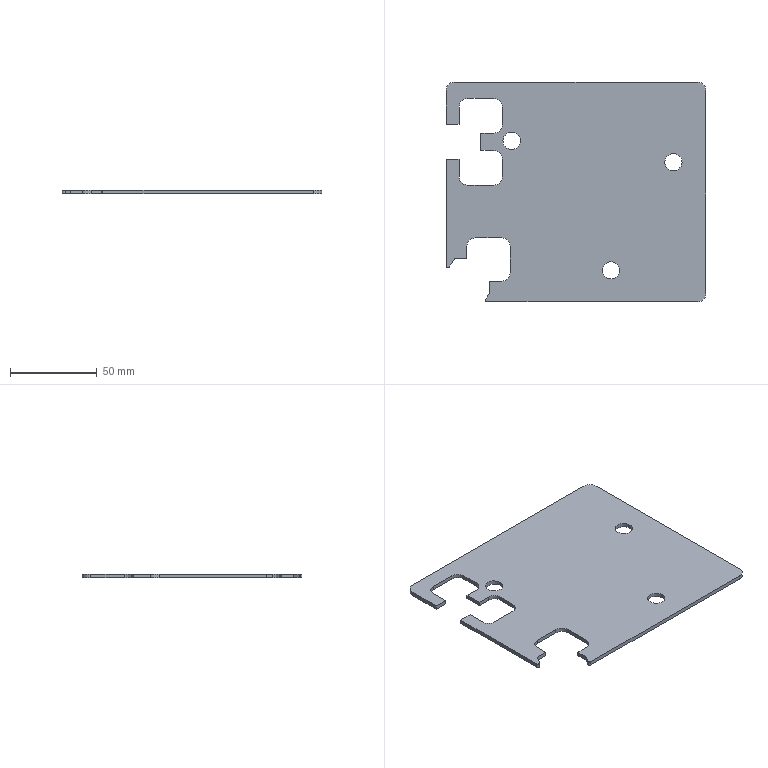Part | SolidWorks | features Fillet 1, FlatPattern 1, SMBaseFlange 1, SheetMetal 1 | 1 solid | 47 faces | box 150 x 127 x 2.3 mm | volume 37985 mm3 | plane 26 | cylinder 21 | commonest cylinder face diameters 10 x18 2 x3
STEP:
#1=CARTESIAN_POINT('',(-83.318,-80.043,2.3));
#2=VERTEX_POINT('',#1);
#3=CARTESIAN_POINT('',(-82.318,-81.043,2.3));
#4=VERTEX_POINT('',#3);
#5=CARTESIAN_POINT('',(-82.318,-80.043,2.3));
#6=DIRECTION('',(0.,0.,1.));
#7=DIRECTION('',(-1.,0.,0.));
#8=AXIS2_PLACEMENT_3D('',#5,#6,#7);
#9=CIRCLE('',#8,1.);
#10=EDGE_CURVE('',#2,#4,#9,.T.);
#11=ORIENTED_EDGE('',*,*,#10,.F.);
#12=CARTESIAN_POINT('',(-83.318,-80.043,0.));
#13=VERTEX_POINT('',#12);
#14=CARTESIAN_POINT('',(-83.318,-80.043,2.3));
#15=DIRECTION('',(0.,0.,-1.));
#16=VECTOR('',#15,1000.);
#17=LINE('',#14,#16);
#18=EDGE_CURVE('',#2,#13,#17,.T.);
#19=ORIENTED_EDGE('',*,*,#18,.T.);
#20=CARTESIAN_POINT('',(-82.318,-81.043,0.));
#21=VERTEX_POINT('',#20);
#22=CARTESIAN_POINT('',(-82.318,-80.043,0.));
#23=DIRECTION('',(0.,0.,-1.));
#24=DIRECTION('',(-1.,0.,0.));
#25=AXIS2_PLACEMENT_3D('',#22,#23,#24);
#26=CIRCLE('',#25,1.);
#27=EDGE_CURVE('',#21,#13,#26,.T.);
#28=ORIENTED_EDGE('',*,*,#27,.F.);
#29=CARTESIAN_POINT('',(-82.318,-81.043,2.3));
#30=DIRECTION('',(0.,0.,-1.));
#31=VECTOR('',#30,1000.);
#32=LINE('',#29,#31);
#33=EDGE_CURVE('',#4,#21,#32,.T.);
#34=ORIENTED_EDGE('',*,*,#33,.F.);
#35=EDGE_LOOP('',(#11,#19,#28,#34));
#36=FACE_OUTER_BOUND('',#35,.T.);
#37=CARTESIAN_POINT('',(-82.318,-80.043,2.3));
#38=DIRECTION('',(0.,0.,-1.));
#39=DIRECTION('',(-1.,0.,0.));
#40=AXIS2_PLACEMENT_3D('',#37,#38,#39);
#41=CYLINDRICAL_SURFACE('',#40,1.);
#42=ADVANCED_FACE('',(#36),#41,.T.);
#43=CARTESIAN_POINT('',(-15.703,-62.806,2.3));
#44=VERTEX_POINT('',#43);
#45=CARTESIAN_POINT('',(-5.703,-62.806,2.3));
#46=VERTEX_POINT('',#45);
#47=CARTESIAN_POINT('',(-10.703,-62.806,2.3));
#48=DIRECTION('',(0.,0.,1.));
#49=DIRECTION('',(1.,0.,0.));
#50=AXIS2_PLACEMENT_3D('',#47,#48,#49);
#51=CIRCLE('',#50,5.);
#52=EDGE_CURVE('',#44,#46,#51,.T.);
#53=ORIENTED_EDGE('',*,*,#52,.T.);
#54=CARTESIAN_POINT('',(-5.703,-62.806,0.));
#55=VERTEX_POINT('',#54);
#56=CARTESIAN_POINT('',(-5.703,-62.806,2.3));
#57=DIRECTION('',(0.,0.,-1.));
#58=VECTOR('',#57,1000.);
#59=LINE('',#56,#58);
#60=EDGE_CURVE('',#46,#55,#59,.T.);
#61=ORIENTED_EDGE('',*,*,#60,.T.);
#62=CARTESIAN_POINT('',(-15.703,-62.806,0.));
#63=VERTEX_POINT('',#62);
#64=CARTESIAN_POINT('',(-10.703,-62.806,0.));
#65=DIRECTION('',(0.,0.,1.));
#66=DIRECTION('',(1.,0.,0.));
#67=AXIS2_PLACEMENT_3D('',#64,#65,#66);
#68=CIRCLE('',#67,5.);
#69=EDGE_CURVE('',#63,#55,#68,.T.);
#70=ORIENTED_EDGE('',*,*,#69,.F.);
#71=CARTESIAN_POINT('',(-15.703,-62.806,2.3));
#72=DIRECTION('',(0.,0.,-1.));
#73=VECTOR('',#72,1000.);
#74=LINE('',#71,#73);
#75=EDGE_CURVE('',#44,#63,#74,.T.);
#76=ORIENTED_EDGE('',*,*,#75,.F.);
#77=EDGE_LOOP('',(#53,#61,#70,#76));
#78=FACE_OUTER_BOUND('',#77,.T.);
#79=CARTESIAN_POINT('',(-10.703,-62.806,2.3));
#80=DIRECTION('',(0.,0.,-1.));
#81=DIRECTION('',(-1.,0.,0.));
#82=AXIS2_PLACEMENT_3D('',#79,#80,#81);
#83=CYLINDRICAL_SURFACE('',#82,5.);
#84=ADVANCED_FACE('',(#78),#83,.F.);
#85=CARTESIAN_POINT('',(20.359,-0.3437,2.3));
#86=VERTEX_POINT('',#85);
#87=CARTESIAN_POINT('',(30.359,-0.3437,2.3));
#88=VERTEX_POINT('',#87);
#89=CARTESIAN_POINT('',(25.359,-0.3437,2.3));
#90=DIRECTION('',(0.,0.,1.));
#91=DIRECTION('',(1.,0.,0.));
#92=AXIS2_PLACEMENT_3D('',#89,#90,#91);
#93=CIRCLE('',#92,5.);
#94=EDGE_CURVE('',#86,#88,#93,.T.);
#95=ORIENTED_EDGE('',*,*,#94,.T.);
#96=CARTESIAN_POINT('',(30.359,-0.3437,0.));
#97=VERTEX_POINT('',#96);
#98=CARTESIAN_POINT('',(30.359,-0.3437,2.3));
#99=DIRECTION('',(0.,0.,-1.));
#100=VECTOR('',#99,1000.);
#101=LINE('',#98,#100);
#102=EDGE_CURVE('',#88,#97,#101,.T.);
#103=ORIENTED_EDGE('',*,*,#102,.T.);
#104=CARTESIAN_POINT('',(20.359,-0.3437,0.));
#105=VERTEX_POINT('',#104);
#106=CARTESIAN_POINT('',(25.359,-0.3437,0.));
#107=DIRECTION('',(0.,0.,1.));
#108=DIRECTION('',(1.,0.,0.));
#109=AXIS2_PLACEMENT_3D('',#106,#107,#108);
#110=CIRCLE('',#109,5.);
#111=EDGE_CURVE('',#105,#97,#110,.T.);
#112=ORIENTED_EDGE('',*,*,#111,.F.);
#113=CARTESIAN_POINT('',(20.359,-0.3437,2.3));
#114=DIRECTION('',(0.,0.,-1.));
#115=VECTOR('',#114,1000.);
#116=LINE('',#113,#115);
#117=EDGE_CURVE('',#86,#105,#116,.T.);
#118=ORIENTED_EDGE('',*,*,#117,.F.);
#119=EDGE_LOOP('',(#95,#103,#112,#118));
#120=FACE_OUTER_BOUND('',#119,.T.);
#121=CARTESIAN_POINT('',(25.359,-0.3437,2.3));
#122=DIRECTION('',(0.,0.,-1.));
#123=DIRECTION('',(-1.,0.,0.));
#124=AXIS2_PLACEMENT_3D('',#121,#122,#123);
#125=CYLINDRICAL_SURFACE('',#124,5.);
#126=ADVANCED_FACE('',(#120),#125,.F.);
#127=CARTESIAN_POINT('',(-73.07,11.957,2.3));
#128=VERTEX_POINT('',#127);
#129=CARTESIAN_POINT('',(-63.07,11.957,2.3));
#130=VERTEX_POINT('',#129);
#131=CARTESIAN_POINT('',(-68.07,11.957,2.3));
#132=DIRECTION('',(0.,0.,1.));
#133=DIRECTION('',(1.,0.,0.));
#134=AXIS2_PLACEMENT_3D('',#131,#132,#133);
#135=CIRCLE('',#134,5.);
#136=EDGE_CURVE('',#128,#130,#135,.T.);
#137=ORIENTED_EDGE('',*,*,#136,.T.);
#138=CARTESIAN_POINT('',(-63.07,11.957,0.));
#139=VERTEX_POINT('',#138);
#140=CARTESIAN_POINT('',(-63.07,11.957,2.3));
#141=DIRECTION('',(0.,0.,-1.));
#142=VECTOR('',#141,1000.);
#143=LINE('',#140,#142);
#144=EDGE_CURVE('',#130,#139,#143,.T.);
#145=ORIENTED_EDGE('',*,*,#144,.T.);
#146=CARTESIAN_POINT('',(-73.07,11.957,0.));
#147=VERTEX_POINT('',#146);
#148=CARTESIAN_POINT('',(-68.07,11.957,0.));
#149=DIRECTION('',(0.,0.,1.));
#150=DIRECTION('',(1.,0.,0.));
#151=AXIS2_PLACEMENT_3D('',#148,#149,#150);
#152=CIRCLE('',#151,5.);
#153=EDGE_CURVE('',#147,#139,#152,.T.);
#154=ORIENTED_EDGE('',*,*,#153,.F.);
#155=CARTESIAN_POINT('',(-73.07,11.957,2.3));
#156=DIRECTION('',(0.,0.,-1.));
#157=VECTOR('',#156,1000.);
#158=LINE('',#155,#157);
#159=EDGE_CURVE('',#128,#147,#158,.T.);
#160=ORIENTED_EDGE('',*,*,#159,.F.);
#161=EDGE_LOOP('',(#137,#145,#154,#160));
#162=FACE_OUTER_BOUND('',#161,.T.);
#163=CARTESIAN_POINT('',(-68.07,11.957,2.3));
#164=DIRECTION('',(0.,0.,-1.));
#165=DIRECTION('',(-1.,0.,0.));
#166=AXIS2_PLACEMENT_3D('',#163,#164,#165);
#167=CYLINDRICAL_SURFACE('',#166,5.);
#168=ADVANCED_FACE('',(#162),#167,.F.);
#169=CARTESIAN_POINT('',(-80.903,-76.043,2.3));
#170=VERTEX_POINT('',#169);
#171=CARTESIAN_POINT('',(-83.155,-79.497,2.3));
#172=VERTEX_POINT('',#171);
#173=CARTESIAN_POINT('',(-84.164,-81.043,2.3));
#174=DIRECTION('',(-0.5463,-0.8376,0.));
#175=VECTOR('',#174,1000.);
#176=LINE('',#173,#175);
#177=EDGE_CURVE('',#170,#172,#176,.T.);
#178=ORIENTED_EDGE('',*,*,#177,.T.);
#179=CARTESIAN_POINT('',(-82.318,-80.043,2.3));
#180=DIRECTION('',(0.,0.,1.));
#181=DIRECTION('',(-1.,0.,0.));
#182=AXIS2_PLACEMENT_3D('',#179,#180,#181);
#183=CIRCLE('',#182,1.);
#184=EDGE_CURVE('',#172,#2,#183,.T.);
#185=ORIENTED_EDGE('',*,*,#184,.T.);
#186=ORIENTED_EDGE('',*,*,#10,.T.);
#187=CARTESIAN_POINT('',(39.097,-81.043,2.3));
#188=VERTEX_POINT('',#187);
#189=CARTESIAN_POINT('',(-80.903,-81.043,2.3));
#190=DIRECTION('',(1.,0.,0.));
#191=VECTOR('',#190,1000.);
#192=LINE('',#189,#191);
#193=EDGE_CURVE('',#4,#188,#192,.T.);
#194=ORIENTED_EDGE('',*,*,#193,.T.);
#195=CARTESIAN_POINT('',(44.097,-76.043,2.3));
#196=VERTEX_POINT('',#195);
#197=CARTESIAN_POINT('',(39.097,-76.043,2.3));
#198=DIRECTION('',(0.,0.,1.));
#199=DIRECTION('',(-1.,0.,0.));
#200=AXIS2_PLACEMENT_3D('',#197,#198,#199);
#201=CIRCLE('',#200,5.);
#202=EDGE_CURVE('',#188,#196,#201,.T.);
#203=ORIENTED_EDGE('',*,*,#202,.T.);
#204=CARTESIAN_POINT('',(44.097,40.957,2.3));
#205=VERTEX_POINT('',#204);
#206=CARTESIAN_POINT('',(44.097,-76.043,2.3));
#207=DIRECTION('',(0.,1.,0.));
#208=VECTOR('',#207,1000.);
#209=LINE('',#206,#208);
#210=EDGE_CURVE('',#196,#205,#209,.T.);
#211=ORIENTED_EDGE('',*,*,#210,.T.);
#212=CARTESIAN_POINT('',(39.097,45.957,2.3));
#213=VERTEX_POINT('',#212);
#214=CARTESIAN_POINT('',(39.097,40.957,2.3));
#215=DIRECTION('',(0.,0.,1.));
#216=DIRECTION('',(1.,0.,0.));
#217=AXIS2_PLACEMENT_3D('',#214,#215,#216);
#218=CIRCLE('',#217,5.);
#219=EDGE_CURVE('',#205,#213,#218,.T.);
#220=ORIENTED_EDGE('',*,*,#219,.T.);
#221=CARTESIAN_POINT('',(-100.903,45.957,2.3));
#222=VERTEX_POINT('',#221);
#223=CARTESIAN_POINT('',(39.097,45.957,2.3));
#224=DIRECTION('',(-1.,0.,0.));
#225=VECTOR('',#224,1000.);
#226=LINE('',#223,#225);
#227=EDGE_CURVE('',#213,#222,#226,.T.);
#228=ORIENTED_EDGE('',*,*,#227,.T.);
#229=CARTESIAN_POINT('',(-105.903,40.957,2.3));
#230=VERTEX_POINT('',#229);
#231=CARTESIAN_POINT('',(-100.903,40.957,2.3));
#232=DIRECTION('',(0.,0.,1.));
#233=DIRECTION('',(1.,0.,0.));
#234=AXIS2_PLACEMENT_3D('',#231,#232,#233);
#235=CIRCLE('',#234,5.);
#236=EDGE_CURVE('',#222,#230,#235,.T.);
#237=ORIENTED_EDGE('',*,*,#236,.T.);
#238=CARTESIAN_POINT('',(-105.903,21.457,2.3));
#239=VERTEX_POINT('',#238);
#240=CARTESIAN_POINT('',(-105.903,40.957,2.3));
#241=DIRECTION('',(0.,-1.,0.));
#242=VECTOR('',#241,1000.);
#243=LINE('',#240,#242);
#244=EDGE_CURVE('',#230,#239,#243,.T.);
#245=ORIENTED_EDGE('',*,*,#244,.T.);
#246=CARTESIAN_POINT('',(-98.403,21.457,2.3));
#247=VERTEX_POINT('',#246);
#248=CARTESIAN_POINT('',(-105.903,21.457,2.3));
#249=DIRECTION('',(1.,0.,0.));
#250=VECTOR('',#249,1000.);
#251=LINE('',#248,#250);
#252=EDGE_CURVE('',#239,#247,#251,.T.);
#253=ORIENTED_EDGE('',*,*,#252,.T.);
#254=CARTESIAN_POINT('',(-98.403,31.457,2.3));
#255=VERTEX_POINT('',#254);
#256=CARTESIAN_POINT('',(-98.403,21.457,2.3));
#257=DIRECTION('',(0.,1.,0.));
#258=VECTOR('',#257,1000.);
#259=LINE('',#256,#258);
#260=EDGE_CURVE('',#247,#255,#259,.T.);
#261=ORIENTED_EDGE('',*,*,#260,.T.);
#262=CARTESIAN_POINT('',(-93.403,36.457,2.3));
#263=VERTEX_POINT('',#262);
#264=CARTESIAN_POINT('',(-93.403,31.457,2.3));
#265=DIRECTION('',(0.,0.,-1.));
#266=DIRECTION('',(-1.,0.,0.));
#267=AXIS2_PLACEMENT_3D('',#264,#265,#266);
#268=CIRCLE('',#267,5.);
#269=EDGE_CURVE('',#255,#263,#268,.T.);
#270=ORIENTED_EDGE('',*,*,#269,.T.);
#271=CARTESIAN_POINT('',(-78.403,36.457,2.3));
#272=VERTEX_POINT('',#271);
#273=CARTESIAN_POINT('',(-93.403,36.457,2.3));
#274=DIRECTION('',(1.,0.,0.));
#275=VECTOR('',#274,1000.);
#276=LINE('',#273,#275);
#277=EDGE_CURVE('',#263,#272,#276,.T.);
#278=ORIENTED_EDGE('',*,*,#277,.T.);
#279=CARTESIAN_POINT('',(-73.403,31.457,2.3));
#280=VERTEX_POINT('',#279);
#281=CARTESIAN_POINT('',(-78.403,31.457,2.3));
#282=DIRECTION('',(0.,0.,-1.));
#283=DIRECTION('',(-1.,0.,0.));
#284=AXIS2_PLACEMENT_3D('',#281,#282,#283);
#285=CIRCLE('',#284,5.);
#286=EDGE_CURVE('',#272,#280,#285,.T.);
#287=ORIENTED_EDGE('',*,*,#286,.T.);
#288=CARTESIAN_POINT('',(-73.403,21.457,2.3));
#289=VERTEX_POINT('',#288);
#290=CARTESIAN_POINT('',(-73.403,31.457,2.3));
#291=DIRECTION('',(0.,-1.,0.));
#292=VECTOR('',#291,1000.);
#293=LINE('',#290,#292);
#294=EDGE_CURVE('',#280,#289,#293,.T.);
#295=ORIENTED_EDGE('',*,*,#294,.T.);
#296=CARTESIAN_POINT('',(-78.403,16.457,2.3));
#297=VERTEX_POINT('',#296);
#298=CARTESIAN_POINT('',(-78.403,21.457,2.3));
#299=DIRECTION('',(0.,0.,-1.));
#300=DIRECTION('',(-1.,0.,0.));
#301=AXIS2_PLACEMENT_3D('',#298,#299,#300);
#302=CIRCLE('',#301,5.);
#303=EDGE_CURVE('',#289,#297,#302,.T.);
#304=ORIENTED_EDGE('',*,*,#303,.T.);
#305=CARTESIAN_POINT('',(-85.903,16.457,2.3));
#306=VERTEX_POINT('',#305);
#307=CARTESIAN_POINT('',(-78.403,16.457,2.3));
#308=DIRECTION('',(-1.,0.,0.));
#309=VECTOR('',#308,1000.);
#310=LINE('',#307,#309);
#311=EDGE_CURVE('',#297,#306,#310,.T.);
#312=ORIENTED_EDGE('',*,*,#311,.T.);
#313=CARTESIAN_POINT('',(-85.903,6.457,2.3));
#314=VERTEX_POINT('',#313);
#315=CARTESIAN_POINT('',(-85.903,16.457,2.3));
#316=DIRECTION('',(0.,-1.,0.));
#317=VECTOR('',#316,1000.);
#318=LINE('',#315,#317);
#319=EDGE_CURVE('',#306,#314,#318,.T.);
#320=ORIENTED_EDGE('',*,*,#319,.T.);
#321=CARTESIAN_POINT('',(-78.403,6.457,2.3));
#322=VERTEX_POINT('',#321);
#323=CARTESIAN_POINT('',(-85.903,6.457,2.3));
#324=DIRECTION('',(1.,0.,0.));
#325=VECTOR('',#324,1000.);
#326=LINE('',#323,#325);
#327=EDGE_CURVE('',#314,#322,#326,.T.);
#328=ORIENTED_EDGE('',*,*,#327,.T.);
#329=CARTESIAN_POINT('',(-73.403,1.457,2.3));
#330=VERTEX_POINT('',#329);
#331=CARTESIAN_POINT('',(-78.403,1.457,2.3));
#332=DIRECTION('',(0.,0.,-1.));
#333=DIRECTION('',(-1.,0.,0.));
#334=AXIS2_PLACEMENT_3D('',#331,#332,#333);
#335=CIRCLE('',#334,5.);
#336=EDGE_CURVE('',#322,#330,#335,.T.);
#337=ORIENTED_EDGE('',*,*,#336,.T.);
#338=CARTESIAN_POINT('',(-73.403,-8.543,2.3));
#339=VERTEX_POINT('',#338);
#340=CARTESIAN_POINT('',(-73.403,1.457,2.3));
#341=DIRECTION('',(0.,-1.,0.));
#342=VECTOR('',#341,1000.);
#343=LINE('',#340,#342);
#344=EDGE_CURVE('',#330,#339,#343,.T.);
#345=ORIENTED_EDGE('',*,*,#344,.T.);
#346=CARTESIAN_POINT('',(-78.403,-13.543,2.3));
#347=VERTEX_POINT('',#346);
#348=CARTESIAN_POINT('',(-78.403,-8.543,2.3));
#349=DIRECTION('',(0.,0.,-1.));
#350=DIRECTION('',(-1.,0.,0.));
#351=AXIS2_PLACEMENT_3D('',#348,#349,#350);
#352=CIRCLE('',#351,5.);
#353=EDGE_CURVE('',#339,#347,#352,.T.);
#354=ORIENTED_EDGE('',*,*,#353,.T.);
#355=CARTESIAN_POINT('',(-93.403,-13.543,2.3));
#356=VERTEX_POINT('',#355);
#357=CARTESIAN_POINT('',(-78.403,-13.543,2.3));
#358=DIRECTION('',(-1.,0.,0.));
#359=VECTOR('',#358,1000.);
#360=LINE('',#357,#359);
#361=EDGE_CURVE('',#347,#356,#360,.T.);
#362=ORIENTED_EDGE('',*,*,#361,.T.);
#363=CARTESIAN_POINT('',(-98.403,-8.543,2.3));
#364=VERTEX_POINT('',#363);
#365=CARTESIAN_POINT('',(-93.403,-8.543,2.3));
#366=DIRECTION('',(0.,0.,-1.));
#367=DIRECTION('',(-1.,0.,0.));
#368=AXIS2_PLACEMENT_3D('',#365,#366,#367);
#369=CIRCLE('',#368,5.);
#370=EDGE_CURVE('',#356,#364,#369,.T.);
#371=ORIENTED_EDGE('',*,*,#370,.T.);
#372=CARTESIAN_POINT('',(-98.403,1.457,2.3));
#373=VERTEX_POINT('',#372);
#374=CARTESIAN_POINT('',(-98.403,-8.543,2.3));
#375=DIRECTION('',(0.,1.,0.));
#376=VECTOR('',#375,1000.);
#377=LINE('',#374,#376);
#378=EDGE_CURVE('',#364,#373,#377,.T.);
#379=ORIENTED_EDGE('',*,*,#378,.T.);
#380=CARTESIAN_POINT('',(-105.903,1.457,2.3));
#381=VERTEX_POINT('',#380);
#382=CARTESIAN_POINT('',(-98.403,1.457,2.3));
#383=DIRECTION('',(-1.,0.,0.));
#384=VECTOR('',#383,1000.);
#385=LINE('',#382,#384);
#386=EDGE_CURVE('',#373,#381,#385,.T.);
#387=ORIENTED_EDGE('',*,*,#386,.T.);
#388=CARTESIAN_POINT('',(-105.903,-60.346,2.3));
#389=VERTEX_POINT('',#388);
#390=CARTESIAN_POINT('',(-105.903,1.457,2.3));
#391=DIRECTION('',(0.,-1.,0.));
#392=VECTOR('',#391,1000.);
#393=LINE('',#390,#392);
#394=EDGE_CURVE('',#381,#389,#393,.T.);
#395=ORIENTED_EDGE('',*,*,#394,.T.);
#396=CARTESIAN_POINT('',(-104.065,-60.892,2.3));
#397=VERTEX_POINT('',#396);
#398=CARTESIAN_POINT('',(-104.903,-60.346,2.3));
#399=DIRECTION('',(0.,0.,1.));
#400=DIRECTION('',(-1.,0.,0.));
#401=AXIS2_PLACEMENT_3D('',#398,#399,#400);
#402=CIRCLE('',#401,1.);
#403=EDGE_CURVE('',#389,#397,#402,.T.);
#404=ORIENTED_EDGE('',*,*,#403,.T.);
#405=CARTESIAN_POINT('',(-100.903,-56.043,2.3));
#406=VERTEX_POINT('',#405);
#407=CARTESIAN_POINT('',(-105.903,-63.71,2.3));
#408=DIRECTION('',(0.5463,0.8376,0.));
#409=VECTOR('',#408,1000.);
#410=LINE('',#407,#409);
#411=EDGE_CURVE('',#397,#406,#410,.T.);
#412=ORIENTED_EDGE('',*,*,#411,.T.);
#413=CARTESIAN_POINT('',(-93.903,-56.043,2.3));
#414=VERTEX_POINT('',#413);
#415=CARTESIAN_POINT('',(-93.903,-56.043,2.3));
#416=DIRECTION('',(1.,0.,0.));
#417=VECTOR('',#416,1000.);
#418=LINE('',#415,#417);
#419=EDGE_CURVE('',#406,#414,#418,.T.);
#420=ORIENTED_EDGE('',*,*,#419,.T.);
#421=CARTESIAN_POINT('',(-93.903,-49.043,2.3));
#422=VERTEX_POINT('',#421);
#423=CARTESIAN_POINT('',(-93.903,-56.043,2.3));
#424=DIRECTION('',(0.,1.,0.));
#425=VECTOR('',#424,1000.);
#426=LINE('',#423,#425);
#427=EDGE_CURVE('',#414,#422,#426,.T.);
#428=ORIENTED_EDGE('',*,*,#427,.T.);
#429=CARTESIAN_POINT('',(-88.903,-44.043,2.3));
#430=VERTEX_POINT('',#429);
#431=CARTESIAN_POINT('',(-88.903,-49.043,2.3));
#432=DIRECTION('',(0.,0.,-1.));
#433=DIRECTION('',(-1.,0.,0.));
#434=AXIS2_PLACEMENT_3D('',#431,#432,#433);
#435=CIRCLE('',#434,5.);
#436=EDGE_CURVE('',#422,#430,#435,.T.);
#437=ORIENTED_EDGE('',*,*,#436,.T.);
#438=CARTESIAN_POINT('',(-73.903,-44.043,2.3));
#439=VERTEX_POINT('',#438);
#440=CARTESIAN_POINT('',(-88.903,-44.043,2.3));
#441=DIRECTION('',(1.,0.,0.));
#442=VECTOR('',#441,1000.);
#443=LINE('',#440,#442);
#444=EDGE_CURVE('',#430,#439,#443,.T.);
#445=ORIENTED_EDGE('',*,*,#444,.T.);
#446=CARTESIAN_POINT('',(-68.903,-49.043,2.3));
#447=VERTEX_POINT('',#446);
#448=CARTESIAN_POINT('',(-73.903,-49.043,2.3));
#449=DIRECTION('',(0.,0.,-1.));
#450=DIRECTION('',(-1.,0.,0.));
#451=AXIS2_PLACEMENT_3D('',#448,#449,#450);
#452=CIRCLE('',#451,5.);
#453=EDGE_CURVE('',#439,#447,#452,.T.);
#454=ORIENTED_EDGE('',*,*,#453,.T.);
#455=CARTESIAN_POINT('',(-68.903,-64.043,2.3));
#456=VERTEX_POINT('',#455);
#457=CARTESIAN_POINT('',(-68.903,-49.043,2.3));
#458=DIRECTION('',(0.,-1.,0.));
#459=VECTOR('',#458,1000.);
#460=LINE('',#457,#459);
#461=EDGE_CURVE('',#447,#456,#460,.T.);
#462=ORIENTED_EDGE('',*,*,#461,.T.);
#463=CARTESIAN_POINT('',(-73.903,-69.043,2.3));
#464=VERTEX_POINT('',#463);
#465=CARTESIAN_POINT('',(-73.903,-64.043,2.3));
#466=DIRECTION('',(0.,0.,-1.));
#467=DIRECTION('',(-1.,0.,0.));
#468=AXIS2_PLACEMENT_3D('',#465,#466,#467);
#469=CIRCLE('',#468,5.);
#470=EDGE_CURVE('',#456,#464,#469,.T.);
#471=ORIENTED_EDGE('',*,*,#470,.T.);
#472=CARTESIAN_POINT('',(-80.903,-69.043,2.3));
#473=VERTEX_POINT('',#472);
#474=CARTESIAN_POINT('',(-73.903,-69.043,2.3));
#475=DIRECTION('',(-1.,0.,0.));
#476=VECTOR('',#475,1000.);
#477=LINE('',#474,#476);
#478=EDGE_CURVE('',#464,#473,#477,.T.);
#479=ORIENTED_EDGE('',*,*,#478,.T.);
#480=CARTESIAN_POINT('',(-80.903,-69.043,2.3));
#481=DIRECTION('',(0.,-1.,0.));
#482=VECTOR('',#481,1000.);
#483=LINE('',#480,#482);
#484=EDGE_CURVE('',#473,#170,#483,.T.);
#485=ORIENTED_EDGE('',*,*,#484,.T.);
#486=EDGE_LOOP('',(#178,#185,#186,#194,#203,#211,#220,#228,#237,#245,#253,#261,#270,#278,#287,#295,#304,#312,#320,#328,#337,#345,#354,#362,#371,#379,#387,#395,#404,#412,#420,#428,#437,#445,#454,#462,#471,#479,#485));
#487=FACE_OUTER_BOUND('',#486,.T.);
#488=ORIENTED_EDGE('',*,*,#136,.F.);
#489=CARTESIAN_POINT('',(-68.07,11.957,2.3));
#490=DIRECTION('',(0.,0.,1.));
#491=DIRECTION('',(1.,0.,0.));
#492=AXIS2_PLACEMENT_3D('',#489,#490,#491);
#493=CIRCLE('',#492,5.);
#494=EDGE_CURVE('',#130,#128,#493,.T.);
#495=ORIENTED_EDGE('',*,*,#494,.F.);
#496=EDGE_LOOP('',(#488,#495));
#497=FACE_BOUND('',#496,.T.);
#498=ORIENTED_EDGE('',*,*,#94,.F.);
#499=CARTESIAN_POINT('',(25.359,-0.3437,2.3));
#500=DIRECTION('',(0.,0.,1.));
#501=DIRECTION('',(1.,0.,0.));
#502=AXIS2_PLACEMENT_3D('',#499,#500,#501);
#503=CIRCLE('',#502,5.);
#504=EDGE_CURVE('',#88,#86,#503,.T.);
#505=ORIENTED_EDGE('',*,*,#504,.F.);
#506=EDGE_LOOP('',(#498,#505));
#507=FACE_BOUND('',#506,.T.);
#508=ORIENTED_EDGE('',*,*,#52,.F.);
#509=CARTESIAN_POINT('',(-10.703,-62.806,2.3));
#510=DIRECTION('',(0.,0.,1.));
#511=DIRECTION('',(1.,0.,0.));
#512=AXIS2_PLACEMENT_3D('',#509,#510,#511);
#513=CIRCLE('',#512,5.);
#514=EDGE_CURVE('',#46,#44,#513,.T.);
#515=ORIENTED_EDGE('',*,*,#514,.F.);
#516=EDGE_LOOP('',(#508,#515));
#517=FACE_BOUND('',#516,.T.);
#518=CARTESIAN_POINT('',(-93.403,31.457,2.3));
#519=DIRECTION('',(0.,0.,-1.));
#520=DIRECTION('',(-1.,0.,0.));
#521=AXIS2_PLACEMENT_3D('',#518,#519,#520);
#522=PLANE('',#521);
#523=ADVANCED_FACE('',(#487,#497,#507,#517),#522,.F.);
#524=ORIENTED_EDGE('',*,*,#111,.T.);
#525=CARTESIAN_POINT('',(25.359,-0.3437,0.));
#526=DIRECTION('',(0.,0.,1.));
#527=DIRECTION('',(1.,0.,0.));
#528=AXIS2_PLACEMENT_3D('',#525,#526,#527);
#529=CIRCLE('',#528,5.);
#530=EDGE_CURVE('',#97,#105,#529,.T.);
#531=ORIENTED_EDGE('',*,*,#530,.T.);
#532=EDGE_LOOP('',(#524,#531));
#533=FACE_BOUND('',#532,.T.);
#534=CARTESIAN_POINT('',(39.097,-81.043,0.));
#535=VERTEX_POINT('',#534);
#536=CARTESIAN_POINT('',(-80.903,-81.043,0.));
#537=DIRECTION('',(1.,0.,0.));
#538=VECTOR('',#537,1000.);
#539=LINE('',#536,#538);
#540=EDGE_CURVE('',#21,#535,#539,.T.);
#541=ORIENTED_EDGE('',*,*,#540,.F.);
#542=ORIENTED_EDGE('',*,*,#27,.T.);
#543=CARTESIAN_POINT('',(-83.155,-79.497,0.));
#544=VERTEX_POINT('',#543);
#545=CARTESIAN_POINT('',(-82.318,-80.043,0.));
#546=DIRECTION('',(0.,0.,-1.));
#547=DIRECTION('',(-1.,0.,0.));
#548=AXIS2_PLACEMENT_3D('',#545,#546,#547);
#549=CIRCLE('',#548,1.);
#550=EDGE_CURVE('',#13,#544,#549,.T.);
#551=ORIENTED_EDGE('',*,*,#550,.T.);
#552=CARTESIAN_POINT('',(-80.903,-76.043,0.));
#553=VERTEX_POINT('',#552);
#554=CARTESIAN_POINT('',(-84.164,-81.043,0.));
#555=DIRECTION('',(-0.5463,-0.8376,0.));
#556=VECTOR('',#555,1000.);
#557=LINE('',#554,#556);
#558=EDGE_CURVE('',#553,#544,#557,.T.);
#559=ORIENTED_EDGE('',*,*,#558,.F.);
#560=CARTESIAN_POINT('',(-80.903,-69.043,0.));
#561=VERTEX_POINT('',#560);
#562=CARTESIAN_POINT('',(-80.903,-69.043,0.));
#563=DIRECTION('',(0.,-1.,0.));
#564=VECTOR('',#563,1000.);
#565=LINE('',#562,#564);
#566=EDGE_CURVE('',#561,#553,#565,.T.);
#567=ORIENTED_EDGE('',*,*,#566,.F.);
#568=CARTESIAN_POINT('',(-73.903,-69.043,0.));
#569=VERTEX_POINT('',#568);
#570=CARTESIAN_POINT('',(-73.903,-69.043,0.));
#571=DIRECTION('',(-1.,0.,0.));
#572=VECTOR('',#571,1000.);
#573=LINE('',#570,#572);
#574=EDGE_CURVE('',#569,#561,#573,.T.);
#575=ORIENTED_EDGE('',*,*,#574,.F.);
#576=CARTESIAN_POINT('',(-68.903,-64.043,0.));
#577=VERTEX_POINT('',#576);
#578=CARTESIAN_POINT('',(-73.903,-64.043,0.));
#579=DIRECTION('',(0.,0.,-1.));
#580=DIRECTION('',(-1.,0.,0.));
#581=AXIS2_PLACEMENT_3D('',#578,#579,#580);
#582=CIRCLE('',#581,5.);
#583=EDGE_CURVE('',#577,#569,#582,.T.);
#584=ORIENTED_EDGE('',*,*,#583,.F.);
#585=CARTESIAN_POINT('',(-68.903,-49.043,0.));
#586=VERTEX_POINT('',#585);
#587=CARTESIAN_POINT('',(-68.903,-49.043,0.));
#588=DIRECTION('',(0.,-1.,0.));
#589=VECTOR('',#588,1000.);
#590=LINE('',#587,#589);
#591=EDGE_CURVE('',#586,#577,#590,.T.);
#592=ORIENTED_EDGE('',*,*,#591,.F.);
#593=CARTESIAN_POINT('',(-73.903,-44.043,0.));
#594=VERTEX_POINT('',#593);
#595=CARTESIAN_POINT('',(-73.903,-49.043,0.));
#596=DIRECTION('',(0.,0.,-1.));
#597=DIRECTION('',(-1.,0.,0.));
#598=AXIS2_PLACEMENT_3D('',#595,#596,#597);
#599=CIRCLE('',#598,5.);
#600=EDGE_CURVE('',#594,#586,#599,.T.);
#601=ORIENTED_EDGE('',*,*,#600,.F.);
#602=CARTESIAN_POINT('',(-88.903,-44.043,0.));
#603=VERTEX_POINT('',#602);
#604=CARTESIAN_POINT('',(-88.903,-44.043,0.));
#605=DIRECTION('',(1.,0.,0.));
#606=VECTOR('',#605,1000.);
#607=LINE('',#604,#606);
#608=EDGE_CURVE('',#603,#594,#607,.T.);
#609=ORIENTED_EDGE('',*,*,#608,.F.);
#610=CARTESIAN_POINT('',(-93.903,-49.043,0.));
#611=VERTEX_POINT('',#610);
#612=CARTESIAN_POINT('',(-88.903,-49.043,0.));
#613=DIRECTION('',(0.,0.,-1.));
#614=DIRECTION('',(-1.,0.,0.));
#615=AXIS2_PLACEMENT_3D('',#612,#613,#614);
#616=CIRCLE('',#615,5.);
#617=EDGE_CURVE('',#611,#603,#616,.T.);
#618=ORIENTED_EDGE('',*,*,#617,.F.);
#619=CARTESIAN_POINT('',(-93.903,-56.043,0.));
#620=VERTEX_POINT('',#619);
#621=CARTESIAN_POINT('',(-93.903,-56.043,0.));
#622=DIRECTION('',(0.,1.,0.));
#623=VECTOR('',#622,1000.);
#624=LINE('',#621,#623);
#625=EDGE_CURVE('',#620,#611,#624,.T.);
#626=ORIENTED_EDGE('',*,*,#625,.F.);
#627=CARTESIAN_POINT('',(-100.903,-56.043,0.));
#628=VERTEX_POINT('',#627);
#629=CARTESIAN_POINT('',(-93.903,-56.043,0.));
#630=DIRECTION('',(1.,0.,0.));
#631=VECTOR('',#630,1000.);
#632=LINE('',#629,#631);
#633=EDGE_CURVE('',#628,#620,#632,.T.);
#634=ORIENTED_EDGE('',*,*,#633,.F.);
#635=CARTESIAN_POINT('',(-104.065,-60.892,0.));
#636=VERTEX_POINT('',#635);
#637=CARTESIAN_POINT('',(-105.903,-63.71,0.));
#638=DIRECTION('',(0.5463,0.8376,0.));
#639=VECTOR('',#638,1000.);
#640=LINE('',#637,#639);
#641=EDGE_CURVE('',#636,#628,#640,.T.);
#642=ORIENTED_EDGE('',*,*,#641,.F.);
#643=CARTESIAN_POINT('',(-105.903,-60.346,0.));
#644=VERTEX_POINT('',#643);
#645=CARTESIAN_POINT('',(-104.903,-60.346,0.));
#646=DIRECTION('',(0.,0.,-1.));
#647=DIRECTION('',(-1.,0.,0.));
#648=AXIS2_PLACEMENT_3D('',#645,#646,#647);
#649=CIRCLE('',#648,1.);
#650=EDGE_CURVE('',#636,#644,#649,.T.);
#651=ORIENTED_EDGE('',*,*,#650,.T.);
#652=CARTESIAN_POINT('',(-105.903,1.457,0.));
#653=VERTEX_POINT('',#652);
#654=CARTESIAN_POINT('',(-105.903,-56.043,0.));
#655=DIRECTION('',(0.,-1.,0.));
#656=VECTOR('',#655,1000.);
#657=LINE('',#654,#656);
#658=EDGE_CURVE('',#653,#644,#657,.T.);
#659=ORIENTED_EDGE('',*,*,#658,.F.);
#660=CARTESIAN_POINT('',(-98.403,1.457,0.));
#661=VERTEX_POINT('',#660);
#662=CARTESIAN_POINT('',(-98.403,1.457,0.));
#663=DIRECTION('',(-1.,0.,0.));
#664=VECTOR('',#663,1000.);
#665=LINE('',#662,#664);
#666=EDGE_CURVE('',#661,#653,#665,.T.);
#667=ORIENTED_EDGE('',*,*,#666,.F.);
#668=CARTESIAN_POINT('',(-98.403,-8.543,0.));
#669=VERTEX_POINT('',#668);
#670=CARTESIAN_POINT('',(-98.403,-8.543,0.));
#671=DIRECTION('',(0.,1.,0.));
#672=VECTOR('',#671,1000.);
#673=LINE('',#670,#672);
#674=EDGE_CURVE('',#669,#661,#673,.T.);
#675=ORIENTED_EDGE('',*,*,#674,.F.);
#676=CARTESIAN_POINT('',(-93.403,-13.543,0.));
#677=VERTEX_POINT('',#676);
#678=CARTESIAN_POINT('',(-93.403,-8.543,0.));
#679=DIRECTION('',(0.,0.,-1.));
#680=DIRECTION('',(-1.,0.,0.));
#681=AXIS2_PLACEMENT_3D('',#678,#679,#680);
#682=CIRCLE('',#681,5.);
#683=EDGE_CURVE('',#677,#669,#682,.T.);
#684=ORIENTED_EDGE('',*,*,#683,.F.);
#685=CARTESIAN_POINT('',(-78.403,-13.543,0.));
#686=VERTEX_POINT('',#685);
#687=CARTESIAN_POINT('',(-78.403,-13.543,0.));
#688=DIRECTION('',(-1.,0.,0.));
#689=VECTOR('',#688,1000.);
#690=LINE('',#687,#689);
#691=EDGE_CURVE('',#686,#677,#690,.T.);
#692=ORIENTED_EDGE('',*,*,#691,.F.);
#693=CARTESIAN_POINT('',(-73.403,-8.543,0.));
#694=VERTEX_POINT('',#693);
#695=CARTESIAN_POINT('',(-78.403,-8.543,0.));
#696=DIRECTION('',(0.,0.,-1.));
#697=DIRECTION('',(-1.,0.,0.));
#698=AXIS2_PLACEMENT_3D('',#695,#696,#697);
#699=CIRCLE('',#698,5.);
#700=EDGE_CURVE('',#694,#686,#699,.T.);
#701=ORIENTED_EDGE('',*,*,#700,.F.);
#702=CARTESIAN_POINT('',(-73.403,1.457,0.));
#703=VERTEX_POINT('',#702);
#704=CARTESIAN_POINT('',(-73.403,1.457,0.));
#705=DIRECTION('',(0.,-1.,0.));
#706=VECTOR('',#705,1000.);
#707=LINE('',#704,#706);
#708=EDGE_CURVE('',#703,#694,#707,.T.);
#709=ORIENTED_EDGE('',*,*,#708,.F.);
#710=CARTESIAN_POINT('',(-78.403,6.457,0.));
#711=VERTEX_POINT('',#710);
#712=CARTESIAN_POINT('',(-78.403,1.457,0.));
#713=DIRECTION('',(0.,0.,-1.));
#714=DIRECTION('',(-1.,0.,0.));
#715=AXIS2_PLACEMENT_3D('',#712,#713,#714);
#716=CIRCLE('',#715,5.);
#717=EDGE_CURVE('',#711,#703,#716,.T.);
#718=ORIENTED_EDGE('',*,*,#717,.F.);
#719=CARTESIAN_POINT('',(-85.903,6.457,0.));
#720=VERTEX_POINT('',#719);
#721=CARTESIAN_POINT('',(-85.903,6.457,0.));
#722=DIRECTION('',(1.,0.,0.));
#723=VECTOR('',#722,1000.);
#724=LINE('',#721,#723);
#725=EDGE_CURVE('',#720,#711,#724,.T.);
#726=ORIENTED_EDGE('',*,*,#725,.F.);
#727=CARTESIAN_POINT('',(-85.903,16.457,0.));
#728=VERTEX_POINT('',#727);
#729=CARTESIAN_POINT('',(-85.903,16.457,0.));
#730=DIRECTION('',(0.,-1.,0.));
#731=VECTOR('',#730,1000.);
#732=LINE('',#729,#731);
#733=EDGE_CURVE('',#728,#720,#732,.T.);
#734=ORIENTED_EDGE('',*,*,#733,.F.);
#735=CARTESIAN_POINT('',(-78.403,16.457,0.));
#736=VERTEX_POINT('',#735);
#737=CARTESIAN_POINT('',(-78.403,16.457,0.));
#738=DIRECTION('',(-1.,0.,0.));
#739=VECTOR('',#738,1000.);
#740=LINE('',#737,#739);
#741=EDGE_CURVE('',#736,#728,#740,.T.);
#742=ORIENTED_EDGE('',*,*,#741,.F.);
#743=CARTESIAN_POINT('',(-73.403,21.457,0.));
#744=VERTEX_POINT('',#743);
#745=CARTESIAN_POINT('',(-78.403,21.457,0.));
#746=DIRECTION('',(0.,0.,-1.));
#747=DIRECTION('',(-1.,0.,0.));
#748=AXIS2_PLACEMENT_3D('',#745,#746,#747);
#749=CIRCLE('',#748,5.);
#750=EDGE_CURVE('',#744,#736,#749,.T.);
#751=ORIENTED_EDGE('',*,*,#750,.F.);
#752=CARTESIAN_POINT('',(-73.403,31.457,0.));
#753=VERTEX_POINT('',#752);
#754=CARTESIAN_POINT('',(-73.403,31.457,0.));
#755=DIRECTION('',(0.,-1.,0.));
#756=VECTOR('',#755,1000.);
#757=LINE('',#754,#756);
#758=EDGE_CURVE('',#753,#744,#757,.T.);
#759=ORIENTED_EDGE('',*,*,#758,.F.);
#760=CARTESIAN_POINT('',(-78.403,36.457,0.));
#761=VERTEX_POINT('',#760);
#762=CARTESIAN_POINT('',(-78.403,31.457,0.));
#763=DIRECTION('',(0.,0.,-1.));
#764=DIRECTION('',(-1.,0.,0.));
#765=AXIS2_PLACEMENT_3D('',#762,#763,#764);
#766=CIRCLE('',#765,5.);
#767=EDGE_CURVE('',#761,#753,#766,.T.);
#768=ORIENTED_EDGE('',*,*,#767,.F.);
#769=CARTESIAN_POINT('',(-93.403,36.457,0.));
#770=VERTEX_POINT('',#769);
#771=CARTESIAN_POINT('',(-93.403,36.457,0.));
#772=DIRECTION('',(1.,0.,0.));
#773=VECTOR('',#772,1000.);
#774=LINE('',#771,#773);
#775=EDGE_CURVE('',#770,#761,#774,.T.);
#776=ORIENTED_EDGE('',*,*,#775,.F.);
#777=CARTESIAN_POINT('',(-98.403,31.457,0.));
#778=VERTEX_POINT('',#777);
#779=CARTESIAN_POINT('',(-93.403,31.457,0.));
#780=DIRECTION('',(0.,0.,-1.));
#781=DIRECTION('',(-1.,0.,0.));
#782=AXIS2_PLACEMENT_3D('',#779,#780,#781);
#783=CIRCLE('',#782,5.);
#784=EDGE_CURVE('',#778,#770,#783,.T.);
#785=ORIENTED_EDGE('',*,*,#784,.F.);
#786=CARTESIAN_POINT('',(-98.403,21.457,0.));
#787=VERTEX_POINT('',#786);
#788=CARTESIAN_POINT('',(-98.403,21.457,0.));
#789=DIRECTION('',(0.,1.,0.));
#790=VECTOR('',#789,1000.);
#791=LINE('',#788,#790);
#792=EDGE_CURVE('',#787,#778,#791,.T.);
#793=ORIENTED_EDGE('',*,*,#792,.F.);
#794=CARTESIAN_POINT('',(-105.903,21.457,0.));
#795=VERTEX_POINT('',#794);
#796=CARTESIAN_POINT('',(-105.903,21.457,0.));
#797=DIRECTION('',(1.,0.,0.));
#798=VECTOR('',#797,1000.);
#799=LINE('',#796,#798);
#800=EDGE_CURVE('',#795,#787,#799,.T.);
#801=ORIENTED_EDGE('',*,*,#800,.F.);
#802=CARTESIAN_POINT('',(-105.903,40.957,0.));
#803=VERTEX_POINT('',#802);
#804=CARTESIAN_POINT('',(-105.903,40.957,0.));
#805=DIRECTION('',(0.,-1.,0.));
#806=VECTOR('',#805,1000.);
#807=LINE('',#804,#806);
#808=EDGE_CURVE('',#803,#795,#807,.T.);
#809=ORIENTED_EDGE('',*,*,#808,.F.);
#810=CARTESIAN_POINT('',(-100.903,45.957,0.));
#811=VERTEX_POINT('',#810);
#812=CARTESIAN_POINT('',(-100.903,40.957,0.));
#813=DIRECTION('',(0.,0.,1.));
#814=DIRECTION('',(1.,0.,0.));
#815=AXIS2_PLACEMENT_3D('',#812,#813,#814);
#816=CIRCLE('',#815,5.);
#817=EDGE_CURVE('',#811,#803,#816,.T.);
#818=ORIENTED_EDGE('',*,*,#817,.F.);
#819=CARTESIAN_POINT('',(39.097,45.957,0.));
#820=VERTEX_POINT('',#819);
#821=CARTESIAN_POINT('',(39.097,45.957,0.));
#822=DIRECTION('',(-1.,0.,0.));
#823=VECTOR('',#822,1000.);
#824=LINE('',#821,#823);
#825=EDGE_CURVE('',#820,#811,#824,.T.);
#826=ORIENTED_EDGE('',*,*,#825,.F.);
#827=CARTESIAN_POINT('',(44.097,40.957,0.));
#828=VERTEX_POINT('',#827);
#829=CARTESIAN_POINT('',(39.097,40.957,0.));
#830=DIRECTION('',(0.,0.,1.));
#831=DIRECTION('',(1.,0.,0.));
#832=AXIS2_PLACEMENT_3D('',#829,#830,#831);
#833=CIRCLE('',#832,5.);
#834=EDGE_CURVE('',#828,#820,#833,.T.);
#835=ORIENTED_EDGE('',*,*,#834,.F.);
#836=CARTESIAN_POINT('',(44.097,-76.043,0.));
#837=VERTEX_POINT('',#836);
#838=CARTESIAN_POINT('',(44.097,-76.043,0.));
#839=DIRECTION('',(0.,1.,0.));
#840=VECTOR('',#839,1000.);
#841=LINE('',#838,#840);
#842=EDGE_CURVE('',#837,#828,#841,.T.);
#843=ORIENTED_EDGE('',*,*,#842,.F.);
#844=CARTESIAN_POINT('',(39.097,-76.043,0.));
#845=DIRECTION('',(0.,0.,1.));
#846=DIRECTION('',(-1.,0.,0.));
#847=AXIS2_PLACEMENT_3D('',#844,#845,#846);
#848=CIRCLE('',#847,5.);
#849=EDGE_CURVE('',#535,#837,#848,.T.);
#850=ORIENTED_EDGE('',*,*,#849,.F.);
#851=EDGE_LOOP('',(#541,#542,#551,#559,#567,#575,#584,#592,#601,#609,#618,#626,#634,#642,#651,#659,#667,#675,#684,#692,#701,#709,#718,#726,#734,#742,#751,#759,#768,#776,#785,#793,#801,#809,#818,#826,#835,#843,#850));
#852=FACE_OUTER_BOUND('',#851,.T.);
#853=ORIENTED_EDGE('',*,*,#153,.T.);
#854=CARTESIAN_POINT('',(-68.07,11.957,0.));
#855=DIRECTION('',(0.,0.,1.));
#856=DIRECTION('',(1.,0.,0.));
#857=AXIS2_PLACEMENT_3D('',#854,#855,#856);
#858=CIRCLE('',#857,5.);
#859=EDGE_CURVE('',#139,#147,#858,.T.);
#860=ORIENTED_EDGE('',*,*,#859,.T.);
#861=EDGE_LOOP('',(#853,#860));
#862=FACE_BOUND('',#861,.T.);
#863=ORIENTED_EDGE('',*,*,#69,.T.);
#864=CARTESIAN_POINT('',(-10.703,-62.806,0.));
#865=DIRECTION('',(0.,0.,1.));
#866=DIRECTION('',(1.,0.,0.));
#867=AXIS2_PLACEMENT_3D('',#864,#865,#866);
#868=CIRCLE('',#867,5.);
#869=EDGE_CURVE('',#55,#63,#868,.T.);
#870=ORIENTED_EDGE('',*,*,#869,.T.);
#871=EDGE_LOOP('',(#863,#870));
#872=FACE_BOUND('',#871,.T.);
#873=CARTESIAN_POINT('',(-93.403,31.457,0.));
#874=DIRECTION('',(0.,0.,-1.));
#875=DIRECTION('',(-1.,0.,0.));
#876=AXIS2_PLACEMENT_3D('',#873,#874,#875);
#877=PLANE('',#876);
#878=ADVANCED_FACE('',(#533,#852,#862,#872),#877,.T.);
#879=ORIENTED_EDGE('',*,*,#792,.T.);
#880=CARTESIAN_POINT('',(-98.403,31.457,2.3));
#881=DIRECTION('',(0.,0.,-1.));
#882=VECTOR('',#881,1000.);
#883=LINE('',#880,#882);
#884=EDGE_CURVE('',#255,#778,#883,.T.);
#885=ORIENTED_EDGE('',*,*,#884,.F.);
#886=ORIENTED_EDGE('',*,*,#260,.F.);
#887=CARTESIAN_POINT('',(-98.403,21.457,2.3));
#888=DIRECTION('',(0.,0.,-1.));
#889=VECTOR('',#888,1000.);
#890=LINE('',#887,#889);
#891=EDGE_CURVE('',#247,#787,#890,.T.);
#892=ORIENTED_EDGE('',*,*,#891,.T.);
#893=EDGE_LOOP('',(#879,#885,#886,#892));
#894=FACE_OUTER_BOUND('',#893,.T.);
#895=CARTESIAN_POINT('',(-98.403,21.457,2.3));
#896=DIRECTION('',(-1.,0.,0.));
#897=DIRECTION('',(0.,0.,1.));
#898=AXIS2_PLACEMENT_3D('',#895,#896,#897);
#899=PLANE('',#898);
#900=ADVANCED_FACE('',(#894),#899,.F.);
#901=ORIENTED_EDGE('',*,*,#784,.T.);
#902=CARTESIAN_POINT('',(-93.403,36.457,2.3));
#903=DIRECTION('',(0.,0.,-1.));
#904=VECTOR('',#903,1000.);
#905=LINE('',#902,#904);
#906=EDGE_CURVE('',#263,#770,#905,.T.);
#907=ORIENTED_EDGE('',*,*,#906,.F.);
#908=ORIENTED_EDGE('',*,*,#269,.F.);
#909=ORIENTED_EDGE('',*,*,#884,.T.);
#910=EDGE_LOOP('',(#901,#907,#908,#909));
#911=FACE_OUTER_BOUND('',#910,.T.);
#912=CARTESIAN_POINT('',(-93.403,31.457,2.3));
#913=DIRECTION('',(0.,0.,-1.));
#914=DIRECTION('',(-1.,0.,0.));
#915=AXIS2_PLACEMENT_3D('',#912,#913,#914);
#916=CYLINDRICAL_SURFACE('',#915,5.);
#917=ADVANCED_FACE('',(#911),#916,.F.);
#918=ORIENTED_EDGE('',*,*,#775,.T.);
#919=CARTESIAN_POINT('',(-78.403,36.457,2.3));
#920=DIRECTION('',(0.,0.,-1.));
#921=VECTOR('',#920,1000.);
#922=LINE('',#919,#921);
#923=EDGE_CURVE('',#272,#761,#922,.T.);
#924=ORIENTED_EDGE('',*,*,#923,.F.);
#925=ORIENTED_EDGE('',*,*,#277,.F.);
#926=ORIENTED_EDGE('',*,*,#906,.T.);
#927=EDGE_LOOP('',(#918,#924,#925,#926));
#928=FACE_OUTER_BOUND('',#927,.T.);
#929=CARTESIAN_POINT('',(-93.403,36.457,2.3));
#930=DIRECTION('',(0.,1.,0.));
#931=DIRECTION('',(-1.,0.,0.));
#932=AXIS2_PLACEMENT_3D('',#929,#930,#931);
#933=PLANE('',#932);
#934=ADVANCED_FACE('',(#928),#933,.F.);
#935=ORIENTED_EDGE('',*,*,#767,.T.);
#936=CARTESIAN_POINT('',(-73.403,31.457,2.3));
#937=DIRECTION('',(0.,0.,-1.));
#938=VECTOR('',#937,1000.);
#939=LINE('',#936,#938);
#940=EDGE_CURVE('',#280,#753,#939,.T.);
#941=ORIENTED_EDGE('',*,*,#940,.F.);
#942=ORIENTED_EDGE('',*,*,#286,.F.);
#943=ORIENTED_EDGE('',*,*,#923,.T.);
#944=EDGE_LOOP('',(#935,#941,#942,#943));
#945=FACE_OUTER_BOUND('',#944,.T.);
#946=CARTESIAN_POINT('',(-78.403,31.457,2.3));
#947=DIRECTION('',(0.,0.,-1.));
#948=DIRECTION('',(-1.,0.,0.));
#949=AXIS2_PLACEMENT_3D('',#946,#947,#948);
#950=CYLINDRICAL_SURFACE('',#949,5.);
#951=ADVANCED_FACE('',(#945),#950,.F.);
#952=ORIENTED_EDGE('',*,*,#758,.T.);
#953=CARTESIAN_POINT('',(-73.403,21.457,2.3));
#954=DIRECTION('',(0.,0.,-1.));
#955=VECTOR('',#954,1000.);
#956=LINE('',#953,#955);
#957=EDGE_CURVE('',#289,#744,#956,.T.);
#958=ORIENTED_EDGE('',*,*,#957,.F.);
#959=ORIENTED_EDGE('',*,*,#294,.F.);
#960=ORIENTED_EDGE('',*,*,#940,.T.);
#961=EDGE_LOOP('',(#952,#958,#959,#960));
#962=FACE_OUTER_BOUND('',#961,.T.);
#963=CARTESIAN_POINT('',(-73.403,31.457,2.3));
#964=DIRECTION('',(1.,0.,0.));
#965=DIRECTION('',(0.,0.,-1.));
#966=AXIS2_PLACEMENT_3D('',#963,#964,#965);
#967=PLANE('',#966);
#968=ADVANCED_FACE('',(#962),#967,.F.);
#969=ORIENTED_EDGE('',*,*,#750,.T.);
#970=CARTESIAN_POINT('',(-78.403,16.457,2.3));
#971=DIRECTION('',(0.,0.,-1.));
#972=VECTOR('',#971,1000.);
#973=LINE('',#970,#972);
#974=EDGE_CURVE('',#297,#736,#973,.T.);
#975=ORIENTED_EDGE('',*,*,#974,.F.);
#976=ORIENTED_EDGE('',*,*,#303,.F.);
#977=ORIENTED_EDGE('',*,*,#957,.T.);
#978=EDGE_LOOP('',(#969,#975,#976,#977));
#979=FACE_OUTER_BOUND('',#978,.T.);
#980=CARTESIAN_POINT('',(-78.403,21.457,2.3));
#981=DIRECTION('',(0.,0.,-1.));
#982=DIRECTION('',(-1.,0.,0.));
#983=AXIS2_PLACEMENT_3D('',#980,#981,#982);
#984=CYLINDRICAL_SURFACE('',#983,5.);
#985=ADVANCED_FACE('',(#979),#984,.F.);
#986=ORIENTED_EDGE('',*,*,#741,.T.);
#987=CARTESIAN_POINT('',(-85.903,16.457,2.3));
#988=DIRECTION('',(0.,0.,-1.));
#989=VECTOR('',#988,1000.);
#990=LINE('',#987,#989);
#991=EDGE_CURVE('',#306,#728,#990,.T.);
#992=ORIENTED_EDGE('',*,*,#991,.F.);
#993=ORIENTED_EDGE('',*,*,#311,.F.);
#994=ORIENTED_EDGE('',*,*,#974,.T.);
#995=EDGE_LOOP('',(#986,#992,#993,#994));
#996=FACE_OUTER_BOUND('',#995,.T.);
#997=CARTESIAN_POINT('',(-78.403,16.457,2.3));
#998=DIRECTION('',(0.,-1.,0.));
#999=DIRECTION('',(0.,0.,-1.));
#1000=AXIS2_PLACEMENT_3D('',#997,#998,#999);
#1001=PLANE('',#1000);
#1002=ADVANCED_FACE('',(#996),#1001,.F.);
#1003=ORIENTED_EDGE('',*,*,#733,.T.);
#1004=CARTESIAN_POINT('',(-85.903,6.457,2.3));
#1005=DIRECTION('',(0.,0.,-1.));
#1006=VECTOR('',#1005,1000.);
#1007=LINE('',#1004,#1006);
#1008=EDGE_CURVE('',#314,#720,#1007,.T.);
#1009=ORIENTED_EDGE('',*,*,#1008,.F.);
#1010=ORIENTED_EDGE('',*,*,#319,.F.);
#1011=ORIENTED_EDGE('',*,*,#991,.T.);
#1012=EDGE_LOOP('',(#1003,#1009,#1010,#1011));
#1013=FACE_OUTER_BOUND('',#1012,.T.);
#1014=CARTESIAN_POINT('',(-85.903,16.457,2.3));
#1015=DIRECTION('',(1.,0.,0.));
#1016=DIRECTION('',(0.,0.,-1.));
#1017=AXIS2_PLACEMENT_3D('',#1014,#1015,#1016);
#1018=PLANE('',#1017);
#1019=ADVANCED_FACE('',(#1013),#1018,.F.);
#1020=ORIENTED_EDGE('',*,*,#725,.T.);
#1021=CARTESIAN_POINT('',(-78.403,6.457,2.3));
#1022=DIRECTION('',(0.,0.,-1.));
#1023=VECTOR('',#1022,1000.);
#1024=LINE('',#1021,#1023);
#1025=EDGE_CURVE('',#322,#711,#1024,.T.);
#1026=ORIENTED_EDGE('',*,*,#1025,.F.);
#1027=ORIENTED_EDGE('',*,*,#327,.F.);
#1028=ORIENTED_EDGE('',*,*,#1008,.T.);
#1029=EDGE_LOOP('',(#1020,#1026,#1027,#1028));
#1030=FACE_OUTER_BOUND('',#1029,.T.);
#1031=CARTESIAN_POINT('',(-85.903,6.457,2.3));
#1032=DIRECTION('',(0.,1.,0.));
#1033=DIRECTION('',(0.,0.,1.));
#1034=AXIS2_PLACEMENT_3D('',#1031,#1032,#1033);
#1035=PLANE('',#1034);
#1036=ADVANCED_FACE('',(#1030),#1035,.F.);
#1037=ORIENTED_EDGE('',*,*,#717,.T.);
#1038=CARTESIAN_POINT('',(-73.403,1.457,2.3));
#1039=DIRECTION('',(0.,0.,-1.));
#1040=VECTOR('',#1039,1000.);
#1041=LINE('',#1038,#1040);
#1042=EDGE_CURVE('',#330,#703,#1041,.T.);
#1043=ORIENTED_EDGE('',*,*,#1042,.F.);
#1044=ORIENTED_EDGE('',*,*,#336,.F.);
#1045=ORIENTED_EDGE('',*,*,#1025,.T.);
#1046=EDGE_LOOP('',(#1037,#1043,#1044,#1045));
#1047=FACE_OUTER_BOUND('',#1046,.T.);
#1048=CARTESIAN_POINT('',(-78.403,1.457,2.3));
#1049=DIRECTION('',(0.,0.,-1.));
#1050=DIRECTION('',(-1.,0.,0.));
#1051=AXIS2_PLACEMENT_3D('',#1048,#1049,#1050);
#1052=CYLINDRICAL_SURFACE('',#1051,5.);
#1053=ADVANCED_FACE('',(#1047),#1052,.F.);
#1054=ORIENTED_EDGE('',*,*,#708,.T.);
#1055=CARTESIAN_POINT('',(-73.403,-8.543,2.3));
#1056=DIRECTION('',(0.,0.,-1.));
#1057=VECTOR('',#1056,1000.);
#1058=LINE('',#1055,#1057);
#1059=EDGE_CURVE('',#339,#694,#1058,.T.);
#1060=ORIENTED_EDGE('',*,*,#1059,.F.);
#1061=ORIENTED_EDGE('',*,*,#344,.F.);
#1062=ORIENTED_EDGE('',*,*,#1042,.T.);
#1063=EDGE_LOOP('',(#1054,#1060,#1061,#1062));
#1064=FACE_OUTER_BOUND('',#1063,.T.);
#1065=CARTESIAN_POINT('',(-73.403,1.457,2.3));
#1066=DIRECTION('',(1.,0.,0.));
#1067=DIRECTION('',(0.,0.,-1.));
#1068=AXIS2_PLACEMENT_3D('',#1065,#1066,#1067);
#1069=PLANE('',#1068);
#1070=ADVANCED_FACE('',(#1064),#1069,.F.);
#1071=ORIENTED_EDGE('',*,*,#700,.T.);
#1072=CARTESIAN_POINT('',(-78.403,-13.543,2.3));
#1073=DIRECTION('',(0.,0.,-1.));
#1074=VECTOR('',#1073,1000.);
#1075=LINE('',#1072,#1074);
#1076=EDGE_CURVE('',#347,#686,#1075,.T.);
#1077=ORIENTED_EDGE('',*,*,#1076,.F.);
#1078=ORIENTED_EDGE('',*,*,#353,.F.);
#1079=ORIENTED_EDGE('',*,*,#1059,.T.);
#1080=EDGE_LOOP('',(#1071,#1077,#1078,#1079));
#1081=FACE_OUTER_BOUND('',#1080,.T.);
#1082=CARTESIAN_POINT('',(-78.403,-8.543,2.3));
#1083=DIRECTION('',(0.,0.,-1.));
#1084=DIRECTION('',(-1.,0.,0.));
#1085=AXIS2_PLACEMENT_3D('',#1082,#1083,#1084);
#1086=CYLINDRICAL_SURFACE('',#1085,5.);
#1087=ADVANCED_FACE('',(#1081),#1086,.F.);
#1088=ORIENTED_EDGE('',*,*,#691,.T.);
#1089=CARTESIAN_POINT('',(-93.403,-13.543,2.3));
#1090=DIRECTION('',(0.,0.,-1.));
#1091=VECTOR('',#1090,1000.);
#1092=LINE('',#1089,#1091);
#1093=EDGE_CURVE('',#356,#677,#1092,.T.);
#1094=ORIENTED_EDGE('',*,*,#1093,.F.);
#1095=ORIENTED_EDGE('',*,*,#361,.F.);
#1096=ORIENTED_EDGE('',*,*,#1076,.T.);
#1097=EDGE_LOOP('',(#1088,#1094,#1095,#1096));
#1098=FACE_OUTER_BOUND('',#1097,.T.);
#1099=CARTESIAN_POINT('',(-78.403,-13.543,2.3));
#1100=DIRECTION('',(0.,-1.,0.));
#1101=DIRECTION('',(0.,0.,-1.));
#1102=AXIS2_PLACEMENT_3D('',#1099,#1100,#1101);
#1103=PLANE('',#1102);
#1104=ADVANCED_FACE('',(#1098),#1103,.F.);
#1105=ORIENTED_EDGE('',*,*,#683,.T.);
#1106=CARTESIAN_POINT('',(-98.403,-8.543,2.3));
#1107=DIRECTION('',(0.,0.,-1.));
#1108=VECTOR('',#1107,1000.);
#1109=LINE('',#1106,#1108);
#1110=EDGE_CURVE('',#364,#669,#1109,.T.);
#1111=ORIENTED_EDGE('',*,*,#1110,.F.);
#1112=ORIENTED_EDGE('',*,*,#370,.F.);
#1113=ORIENTED_EDGE('',*,*,#1093,.T.);
#1114=EDGE_LOOP('',(#1105,#1111,#1112,#1113));
#1115=FACE_OUTER_BOUND('',#1114,.T.);
#1116=CARTESIAN_POINT('',(-93.403,-8.543,2.3));
#1117=DIRECTION('',(0.,0.,-1.));
#1118=DIRECTION('',(-1.,0.,0.));
#1119=AXIS2_PLACEMENT_3D('',#1116,#1117,#1118);
#1120=CYLINDRICAL_SURFACE('',#1119,5.);
#1121=ADVANCED_FACE('',(#1115),#1120,.F.);
#1122=ORIENTED_EDGE('',*,*,#674,.T.);
#1123=CARTESIAN_POINT('',(-98.403,1.457,2.3));
#1124=DIRECTION('',(0.,0.,-1.));
#1125=VECTOR('',#1124,1000.);
#1126=LINE('',#1123,#1125);
#1127=EDGE_CURVE('',#373,#661,#1126,.T.);
#1128=ORIENTED_EDGE('',*,*,#1127,.F.);
#1129=ORIENTED_EDGE('',*,*,#378,.F.);
#1130=ORIENTED_EDGE('',*,*,#1110,.T.);
#1131=EDGE_LOOP('',(#1122,#1128,#1129,#1130));
#1132=FACE_OUTER_BOUND('',#1131,.T.);
#1133=CARTESIAN_POINT('',(-98.403,-8.543,2.3));
#1134=DIRECTION('',(-1.,0.,0.));
#1135=DIRECTION('',(0.,-1.,0.));
#1136=AXIS2_PLACEMENT_3D('',#1133,#1134,#1135);
#1137=PLANE('',#1136);
#1138=ADVANCED_FACE('',(#1132),#1137,.F.);
#1139=ORIENTED_EDGE('',*,*,#666,.T.);
#1140=CARTESIAN_POINT('',(-105.903,1.457,2.3));
#1141=DIRECTION('',(0.,0.,-1.));
#1142=VECTOR('',#1141,1000.);
#1143=LINE('',#1140,#1142);
#1144=EDGE_CURVE('',#381,#653,#1143,.T.);
#1145=ORIENTED_EDGE('',*,*,#1144,.F.);
#1146=ORIENTED_EDGE('',*,*,#386,.F.);
#1147=ORIENTED_EDGE('',*,*,#1127,.T.);
#1148=EDGE_LOOP('',(#1139,#1145,#1146,#1147));
#1149=FACE_OUTER_BOUND('',#1148,.T.);
#1150=CARTESIAN_POINT('',(-98.403,1.457,2.3));
#1151=DIRECTION('',(0.,-1.,0.));
#1152=DIRECTION('',(0.,0.,-1.));
#1153=AXIS2_PLACEMENT_3D('',#1150,#1151,#1152);
#1154=PLANE('',#1153);
#1155=ADVANCED_FACE('',(#1149),#1154,.F.);
#1156=ORIENTED_EDGE('',*,*,#658,.T.);
#1157=CARTESIAN_POINT('',(-105.903,-60.346,2.3));
#1158=DIRECTION('',(0.,0.,1.));
#1159=VECTOR('',#1158,1000.);
#1160=LINE('',#1157,#1159);
#1161=EDGE_CURVE('',#644,#389,#1160,.T.);
#1162=ORIENTED_EDGE('',*,*,#1161,.T.);
#1163=ORIENTED_EDGE('',*,*,#394,.F.);
#1164=ORIENTED_EDGE('',*,*,#1144,.T.);
#1165=EDGE_LOOP('',(#1156,#1162,#1163,#1164));
#1166=FACE_OUTER_BOUND('',#1165,.T.);
#1167=CARTESIAN_POINT('',(-105.903,-56.043,2.3));
#1168=DIRECTION('',(1.,0.,0.));
#1169=DIRECTION('',(0.,1.,0.));
#1170=AXIS2_PLACEMENT_3D('',#1167,#1168,#1169);
#1171=PLANE('',#1170);
#1172=ADVANCED_FACE('',(#1166),#1171,.F.);
#1173=ORIENTED_EDGE('',*,*,#411,.F.);
#1174=CARTESIAN_POINT('',(-104.065,-60.892,2.3));
#1175=DIRECTION('',(0.,0.,-1.));
#1176=VECTOR('',#1175,1000.);
#1177=LINE('',#1174,#1176);
#1178=EDGE_CURVE('',#397,#636,#1177,.T.);
#1179=ORIENTED_EDGE('',*,*,#1178,.T.);
#1180=ORIENTED_EDGE('',*,*,#641,.T.);
#1181=CARTESIAN_POINT('',(-100.903,-56.043,2.3));
#1182=DIRECTION('',(0.,0.,-1.));
#1183=VECTOR('',#1182,1000.);
#1184=LINE('',#1181,#1183);
#1185=EDGE_CURVE('',#406,#628,#1184,.T.);
#1186=ORIENTED_EDGE('',*,*,#1185,.F.);
#1187=EDGE_LOOP('',(#1173,#1179,#1180,#1186));
#1188=FACE_OUTER_BOUND('',#1187,.T.);
#1189=CARTESIAN_POINT('',(-105.903,-63.71,2.3));
#1190=DIRECTION('',(-0.8376,0.5463,0.));
#1191=DIRECTION('',(-0.5463,-0.8376,0.));
#1192=AXIS2_PLACEMENT_3D('',#1189,#1190,#1191);
#1193=PLANE('',#1192);
#1194=ADVANCED_FACE('',(#1188),#1193,.F.);
#1195=ORIENTED_EDGE('',*,*,#633,.T.);
#1196=CARTESIAN_POINT('',(-93.903,-56.043,2.3));
#1197=DIRECTION('',(0.,0.,-1.));
#1198=VECTOR('',#1197,1000.);
#1199=LINE('',#1196,#1198);
#1200=EDGE_CURVE('',#414,#620,#1199,.T.);
#1201=ORIENTED_EDGE('',*,*,#1200,.F.);
#1202=ORIENTED_EDGE('',*,*,#419,.F.);
#1203=ORIENTED_EDGE('',*,*,#1185,.T.);
#1204=EDGE_LOOP('',(#1195,#1201,#1202,#1203));
#1205=FACE_OUTER_BOUND('',#1204,.T.);
#1206=CARTESIAN_POINT('',(-93.903,-56.043,2.3));
#1207=DIRECTION('',(0.,1.,0.));
#1208=DIRECTION('',(-1.,0.,0.));
#1209=AXIS2_PLACEMENT_3D('',#1206,#1207,#1208);
#1210=PLANE('',#1209);
#1211=ADVANCED_FACE('',(#1205),#1210,.F.);
#1212=ORIENTED_EDGE('',*,*,#625,.T.);
#1213=CARTESIAN_POINT('',(-93.903,-49.043,2.3));
#1214=DIRECTION('',(0.,0.,-1.));
#1215=VECTOR('',#1214,1000.);
#1216=LINE('',#1213,#1215);
#1217=EDGE_CURVE('',#422,#611,#1216,.T.);
#1218=ORIENTED_EDGE('',*,*,#1217,.F.);
#1219=ORIENTED_EDGE('',*,*,#427,.F.);
#1220=ORIENTED_EDGE('',*,*,#1200,.T.);
#1221=EDGE_LOOP('',(#1212,#1218,#1219,#1220));
#1222=FACE_OUTER_BOUND('',#1221,.T.);
#1223=CARTESIAN_POINT('',(-93.903,-56.043,2.3));
#1224=DIRECTION('',(-1.,0.,0.));
#1225=DIRECTION('',(0.,0.,1.));
#1226=AXIS2_PLACEMENT_3D('',#1223,#1224,#1225);
#1227=PLANE('',#1226);
#1228=ADVANCED_FACE('',(#1222),#1227,.F.);
#1229=ORIENTED_EDGE('',*,*,#617,.T.);
#1230=CARTESIAN_POINT('',(-88.903,-44.043,2.3));
#1231=DIRECTION('',(0.,0.,-1.));
#1232=VECTOR('',#1231,1000.);
#1233=LINE('',#1230,#1232);
#1234=EDGE_CURVE('',#430,#603,#1233,.T.);
#1235=ORIENTED_EDGE('',*,*,#1234,.F.);
#1236=ORIENTED_EDGE('',*,*,#436,.F.);
#1237=ORIENTED_EDGE('',*,*,#1217,.T.);
#1238=EDGE_LOOP('',(#1229,#1235,#1236,#1237));
#1239=FACE_OUTER_BOUND('',#1238,.T.);
#1240=CARTESIAN_POINT('',(-88.903,-49.043,2.3));
#1241=DIRECTION('',(0.,0.,-1.));
#1242=DIRECTION('',(-1.,0.,0.));
#1243=AXIS2_PLACEMENT_3D('',#1240,#1241,#1242);
#1244=CYLINDRICAL_SURFACE('',#1243,5.);
#1245=ADVANCED_FACE('',(#1239),#1244,.F.);
#1246=ORIENTED_EDGE('',*,*,#608,.T.);
#1247=CARTESIAN_POINT('',(-73.903,-44.043,2.3));
#1248=DIRECTION('',(0.,0.,-1.));
#1249=VECTOR('',#1248,1000.);
#1250=LINE('',#1247,#1249);
#1251=EDGE_CURVE('',#439,#594,#1250,.T.);
#1252=ORIENTED_EDGE('',*,*,#1251,.F.);
#1253=ORIENTED_EDGE('',*,*,#444,.F.);
#1254=ORIENTED_EDGE('',*,*,#1234,.T.);
#1255=EDGE_LOOP('',(#1246,#1252,#1253,#1254));
#1256=FACE_OUTER_BOUND('',#1255,.T.);
#1257=CARTESIAN_POINT('',(-88.903,-44.043,2.3));
#1258=DIRECTION('',(0.,1.,0.));
#1259=DIRECTION('',(0.,0.,1.));
#1260=AXIS2_PLACEMENT_3D('',#1257,#1258,#1259);
#1261=PLANE('',#1260);
#1262=ADVANCED_FACE('',(#1256),#1261,.F.);
#1263=ORIENTED_EDGE('',*,*,#600,.T.);
#1264=CARTESIAN_POINT('',(-68.903,-49.043,2.3));
#1265=DIRECTION('',(0.,0.,-1.));
#1266=VECTOR('',#1265,1000.);
#1267=LINE('',#1264,#1266);
#1268=EDGE_CURVE('',#447,#586,#1267,.T.);
#1269=ORIENTED_EDGE('',*,*,#1268,.F.);
#1270=ORIENTED_EDGE('',*,*,#453,.F.);
#1271=ORIENTED_EDGE('',*,*,#1251,.T.);
#1272=EDGE_LOOP('',(#1263,#1269,#1270,#1271));
#1273=FACE_OUTER_BOUND('',#1272,.T.);
#1274=CARTESIAN_POINT('',(-73.903,-49.043,2.3));
#1275=DIRECTION('',(0.,0.,-1.));
#1276=DIRECTION('',(-1.,0.,0.));
#1277=AXIS2_PLACEMENT_3D('',#1274,#1275,#1276);
#1278=CYLINDRICAL_SURFACE('',#1277,5.);
#1279=ADVANCED_FACE('',(#1273),#1278,.F.);
#1280=ORIENTED_EDGE('',*,*,#591,.T.);
#1281=CARTESIAN_POINT('',(-68.903,-64.043,2.3));
#1282=DIRECTION('',(0.,0.,-1.));
#1283=VECTOR('',#1282,1000.);
#1284=LINE('',#1281,#1283);
#1285=EDGE_CURVE('',#456,#577,#1284,.T.);
#1286=ORIENTED_EDGE('',*,*,#1285,.F.);
#1287=ORIENTED_EDGE('',*,*,#461,.F.);
#1288=ORIENTED_EDGE('',*,*,#1268,.T.);
#1289=EDGE_LOOP('',(#1280,#1286,#1287,#1288));
#1290=FACE_OUTER_BOUND('',#1289,.T.);
#1291=CARTESIAN_POINT('',(-68.903,-49.043,2.3));
#1292=DIRECTION('',(1.,0.,0.));
#1293=DIRECTION('',(0.,0.,-1.));
#1294=AXIS2_PLACEMENT_3D('',#1291,#1292,#1293);
#1295=PLANE('',#1294);
#1296=ADVANCED_FACE('',(#1290),#1295,.F.);
#1297=ORIENTED_EDGE('',*,*,#583,.T.);
#1298=CARTESIAN_POINT('',(-73.903,-69.043,2.3));
#1299=DIRECTION('',(0.,0.,-1.));
#1300=VECTOR('',#1299,1000.);
#1301=LINE('',#1298,#1300);
#1302=EDGE_CURVE('',#464,#569,#1301,.T.);
#1303=ORIENTED_EDGE('',*,*,#1302,.F.);
#1304=ORIENTED_EDGE('',*,*,#470,.F.);
#1305=ORIENTED_EDGE('',*,*,#1285,.T.);
#1306=EDGE_LOOP('',(#1297,#1303,#1304,#1305));
#1307=FACE_OUTER_BOUND('',#1306,.T.);
#1308=CARTESIAN_POINT('',(-73.903,-64.043,2.3));
#1309=DIRECTION('',(0.,0.,-1.));
#1310=DIRECTION('',(-1.,0.,0.));
#1311=AXIS2_PLACEMENT_3D('',#1308,#1309,#1310);
#1312=CYLINDRICAL_SURFACE('',#1311,5.);
#1313=ADVANCED_FACE('',(#1307),#1312,.F.);
#1314=ORIENTED_EDGE('',*,*,#574,.T.);
#1315=CARTESIAN_POINT('',(-80.903,-69.043,2.3));
#1316=DIRECTION('',(0.,0.,-1.));
#1317=VECTOR('',#1316,1000.);
#1318=LINE('',#1315,#1317);
#1319=EDGE_CURVE('',#473,#561,#1318,.T.);
#1320=ORIENTED_EDGE('',*,*,#1319,.F.);
#1321=ORIENTED_EDGE('',*,*,#478,.F.);
#1322=ORIENTED_EDGE('',*,*,#1302,.T.);
#1323=EDGE_LOOP('',(#1314,#1320,#1321,#1322));
#1324=FACE_OUTER_BOUND('',#1323,.T.);
#1325=CARTESIAN_POINT('',(-73.903,-69.043,2.3));
#1326=DIRECTION('',(0.,-1.,0.));
#1327=DIRECTION('',(0.,0.,-1.));
#1328=AXIS2_PLACEMENT_3D('',#1325,#1326,#1327);
#1329=PLANE('',#1328);
#1330=ADVANCED_FACE('',(#1324),#1329,.F.);
#1331=ORIENTED_EDGE('',*,*,#566,.T.);
#1332=CARTESIAN_POINT('',(-80.903,-76.043,2.3));
#1333=DIRECTION('',(0.,0.,-1.));
#1334=VECTOR('',#1333,1000.);
#1335=LINE('',#1332,#1334);
#1336=EDGE_CURVE('',#170,#553,#1335,.T.);
#1337=ORIENTED_EDGE('',*,*,#1336,.F.);
#1338=ORIENTED_EDGE('',*,*,#484,.F.);
#1339=ORIENTED_EDGE('',*,*,#1319,.T.);
#1340=EDGE_LOOP('',(#1331,#1337,#1338,#1339));
#1341=FACE_OUTER_BOUND('',#1340,.T.);
#1342=CARTESIAN_POINT('',(-80.903,-69.043,2.3));
#1343=DIRECTION('',(1.,0.,0.));
#1344=DIRECTION('',(0.,0.,-1.));
#1345=AXIS2_PLACEMENT_3D('',#1342,#1343,#1344);
#1346=PLANE('',#1345);
#1347=ADVANCED_FACE('',(#1341),#1346,.F.);
#1348=ORIENTED_EDGE('',*,*,#558,.T.);
#1349=CARTESIAN_POINT('',(-83.155,-79.497,2.3));
#1350=DIRECTION('',(0.,0.,1.));
#1351=VECTOR('',#1350,1000.);
#1352=LINE('',#1349,#1351);
#1353=EDGE_CURVE('',#544,#172,#1352,.T.);
#1354=ORIENTED_EDGE('',*,*,#1353,.T.);
#1355=ORIENTED_EDGE('',*,*,#177,.F.);
#1356=ORIENTED_EDGE('',*,*,#1336,.T.);
#1357=EDGE_LOOP('',(#1348,#1354,#1355,#1356));
#1358=FACE_OUTER_BOUND('',#1357,.T.);
#1359=CARTESIAN_POINT('',(-84.164,-81.043,2.3));
#1360=DIRECTION('',(0.8376,-0.5463,0.));
#1361=DIRECTION('',(0.5463,0.8376,0.));
#1362=AXIS2_PLACEMENT_3D('',#1359,#1360,#1361);
#1363=PLANE('',#1362);
#1364=ADVANCED_FACE('',(#1358),#1363,.F.);
#1365=ORIENTED_EDGE('',*,*,#193,.F.);
#1366=ORIENTED_EDGE('',*,*,#33,.T.);
#1367=ORIENTED_EDGE('',*,*,#540,.T.);
#1368=CARTESIAN_POINT('',(39.097,-81.043,2.3));
#1369=DIRECTION('',(0.,0.,-1.));
#1370=VECTOR('',#1369,1000.);
#1371=LINE('',#1368,#1370);
#1372=EDGE_CURVE('',#188,#535,#1371,.T.);
#1373=ORIENTED_EDGE('',*,*,#1372,.F.);
#1374=EDGE_LOOP('',(#1365,#1366,#1367,#1373));
#1375=FACE_OUTER_BOUND('',#1374,.T.);
#1376=CARTESIAN_POINT('',(-80.903,-81.043,2.3));
#1377=DIRECTION('',(0.,1.,0.));
#1378=DIRECTION('',(-1.,0.,0.));
#1379=AXIS2_PLACEMENT_3D('',#1376,#1377,#1378);
#1380=PLANE('',#1379);
#1381=ADVANCED_FACE('',(#1375),#1380,.F.);
#1382=ORIENTED_EDGE('',*,*,#849,.T.);
#1383=CARTESIAN_POINT('',(44.097,-76.043,2.3));
#1384=DIRECTION('',(0.,0.,-1.));
#1385=VECTOR('',#1384,1000.);
#1386=LINE('',#1383,#1385);
#1387=EDGE_CURVE('',#196,#837,#1386,.T.);
#1388=ORIENTED_EDGE('',*,*,#1387,.F.);
#1389=ORIENTED_EDGE('',*,*,#202,.F.);
#1390=ORIENTED_EDGE('',*,*,#1372,.T.);
#1391=EDGE_LOOP('',(#1382,#1388,#1389,#1390));
#1392=FACE_OUTER_BOUND('',#1391,.T.);
#1393=CARTESIAN_POINT('',(39.097,-76.043,2.3));
#1394=DIRECTION('',(0.,0.,-1.));
#1395=DIRECTION('',(-1.,0.,0.));
#1396=AXIS2_PLACEMENT_3D('',#1393,#1394,#1395);
#1397=CYLINDRICAL_SURFACE('',#1396,5.);
#1398=ADVANCED_FACE('',(#1392),#1397,.T.);
#1399=ORIENTED_EDGE('',*,*,#842,.T.);
#1400=CARTESIAN_POINT('',(44.097,40.957,2.3));
#1401=DIRECTION('',(0.,0.,-1.));
#1402=VECTOR('',#1401,1000.);
#1403=LINE('',#1400,#1402);
#1404=EDGE_CURVE('',#205,#828,#1403,.T.);
#1405=ORIENTED_EDGE('',*,*,#1404,.F.);
#1406=ORIENTED_EDGE('',*,*,#210,.F.);
#1407=ORIENTED_EDGE('',*,*,#1387,.T.);
#1408=EDGE_LOOP('',(#1399,#1405,#1406,#1407));
#1409=FACE_OUTER_BOUND('',#1408,.T.);
#1410=CARTESIAN_POINT('',(44.097,-76.043,2.3));
#1411=DIRECTION('',(-1.,0.,0.));
#1412=DIRECTION('',(0.,-1.,0.));
#1413=AXIS2_PLACEMENT_3D('',#1410,#1411,#1412);
#1414=PLANE('',#1413);
#1415=ADVANCED_FACE('',(#1409),#1414,.F.);
#1416=ORIENTED_EDGE('',*,*,#834,.T.);
#1417=CARTESIAN_POINT('',(39.097,45.957,2.3));
#1418=DIRECTION('',(0.,0.,-1.));
#1419=VECTOR('',#1418,1000.);
#1420=LINE('',#1417,#1419);
#1421=EDGE_CURVE('',#213,#820,#1420,.T.);
#1422=ORIENTED_EDGE('',*,*,#1421,.F.);
#1423=ORIENTED_EDGE('',*,*,#219,.F.);
#1424=ORIENTED_EDGE('',*,*,#1404,.T.);
#1425=EDGE_LOOP('',(#1416,#1422,#1423,#1424));
#1426=FACE_OUTER_BOUND('',#1425,.T.);
#1427=CARTESIAN_POINT('',(39.097,40.957,2.3));
#1428=DIRECTION('',(0.,0.,-1.));
#1429=DIRECTION('',(-1.,0.,0.));
#1430=AXIS2_PLACEMENT_3D('',#1427,#1428,#1429);
#1431=CYLINDRICAL_SURFACE('',#1430,5.);
#1432=ADVANCED_FACE('',(#1426),#1431,.T.);
#1433=ORIENTED_EDGE('',*,*,#825,.T.);
#1434=CARTESIAN_POINT('',(-100.903,45.957,2.3));
#1435=DIRECTION('',(0.,0.,-1.));
#1436=VECTOR('',#1435,1000.);
#1437=LINE('',#1434,#1436);
#1438=EDGE_CURVE('',#222,#811,#1437,.T.);
#1439=ORIENTED_EDGE('',*,*,#1438,.F.);
#1440=ORIENTED_EDGE('',*,*,#227,.F.);
#1441=ORIENTED_EDGE('',*,*,#1421,.T.);
#1442=EDGE_LOOP('',(#1433,#1439,#1440,#1441));
#1443=FACE_OUTER_BOUND('',#1442,.T.);
#1444=CARTESIAN_POINT('',(39.097,45.957,2.3));
#1445=DIRECTION('',(0.,-1.,0.));
#1446=DIRECTION('',(1.,0.,0.));
#1447=AXIS2_PLACEMENT_3D('',#1444,#1445,#1446);
#1448=PLANE('',#1447);
#1449=ADVANCED_FACE('',(#1443),#1448,.F.);
#1450=ORIENTED_EDGE('',*,*,#817,.T.);
#1451=CARTESIAN_POINT('',(-105.903,40.957,2.3));
#1452=DIRECTION('',(0.,0.,-1.));
#1453=VECTOR('',#1452,1000.);
#1454=LINE('',#1451,#1453);
#1455=EDGE_CURVE('',#230,#803,#1454,.T.);
#1456=ORIENTED_EDGE('',*,*,#1455,.F.);
#1457=ORIENTED_EDGE('',*,*,#236,.F.);
#1458=ORIENTED_EDGE('',*,*,#1438,.T.);
#1459=EDGE_LOOP('',(#1450,#1456,#1457,#1458));
#1460=FACE_OUTER_BOUND('',#1459,.T.);
#1461=CARTESIAN_POINT('',(-100.903,40.957,2.3));
#1462=DIRECTION('',(0.,0.,-1.));
#1463=DIRECTION('',(-1.,0.,0.));
#1464=AXIS2_PLACEMENT_3D('',#1461,#1462,#1463);
#1465=CYLINDRICAL_SURFACE('',#1464,5.);
#1466=ADVANCED_FACE('',(#1460),#1465,.T.);
#1467=ORIENTED_EDGE('',*,*,#808,.T.);
#1468=CARTESIAN_POINT('',(-105.903,21.457,2.3));
#1469=DIRECTION('',(0.,0.,-1.));
#1470=VECTOR('',#1469,1000.);
#1471=LINE('',#1468,#1470);
#1472=EDGE_CURVE('',#239,#795,#1471,.T.);
#1473=ORIENTED_EDGE('',*,*,#1472,.F.);
#1474=ORIENTED_EDGE('',*,*,#244,.F.);
#1475=ORIENTED_EDGE('',*,*,#1455,.T.);
#1476=EDGE_LOOP('',(#1467,#1473,#1474,#1475));
#1477=FACE_OUTER_BOUND('',#1476,.T.);
#1478=CARTESIAN_POINT('',(-105.903,40.957,2.3));
#1479=DIRECTION('',(1.,0.,0.));
#1480=DIRECTION('',(0.,1.,0.));
#1481=AXIS2_PLACEMENT_3D('',#1478,#1479,#1480);
#1482=PLANE('',#1481);
#1483=ADVANCED_FACE('',(#1477),#1482,.F.);
#1484=ORIENTED_EDGE('',*,*,#800,.T.);
#1485=ORIENTED_EDGE('',*,*,#891,.F.);
#1486=ORIENTED_EDGE('',*,*,#252,.F.);
#1487=ORIENTED_EDGE('',*,*,#1472,.T.);
#1488=EDGE_LOOP('',(#1484,#1485,#1486,#1487));
#1489=FACE_OUTER_BOUND('',#1488,.T.);
#1490=CARTESIAN_POINT('',(-105.903,21.457,2.3));
#1491=DIRECTION('',(0.,1.,0.));
#1492=DIRECTION('',(0.,0.,1.));
#1493=AXIS2_PLACEMENT_3D('',#1490,#1491,#1492);
#1494=PLANE('',#1493);
#1495=ADVANCED_FACE('',(#1489),#1494,.F.);
#1496=ORIENTED_EDGE('',*,*,#144,.F.);
#1497=ORIENTED_EDGE('',*,*,#494,.T.);
#1498=ORIENTED_EDGE('',*,*,#159,.T.);
#1499=ORIENTED_EDGE('',*,*,#859,.F.);
#1500=EDGE_LOOP('',(#1496,#1497,#1498,#1499));
#1501=FACE_OUTER_BOUND('',#1500,.T.);
#1502=CARTESIAN_POINT('',(-68.07,11.957,2.3));
#1503=DIRECTION('',(0.,0.,-1.));
#1504=DIRECTION('',(-1.,0.,0.));
#1505=AXIS2_PLACEMENT_3D('',#1502,#1503,#1504);
#1506=CYLINDRICAL_SURFACE('',#1505,5.);
#1507=ADVANCED_FACE('',(#1501),#1506,.F.);
#1508=ORIENTED_EDGE('',*,*,#102,.F.);
#1509=ORIENTED_EDGE('',*,*,#504,.T.);
#1510=ORIENTED_EDGE('',*,*,#117,.T.);
#1511=ORIENTED_EDGE('',*,*,#530,.F.);
#1512=EDGE_LOOP('',(#1508,#1509,#1510,#1511));
#1513=FACE_OUTER_BOUND('',#1512,.T.);
#1514=CARTESIAN_POINT('',(25.359,-0.3437,2.3));
#1515=DIRECTION('',(0.,0.,-1.));
#1516=DIRECTION('',(-1.,0.,0.));
#1517=AXIS2_PLACEMENT_3D('',#1514,#1515,#1516);
#1518=CYLINDRICAL_SURFACE('',#1517,5.);
#1519=ADVANCED_FACE('',(#1513),#1518,.F.);
#1520=ORIENTED_EDGE('',*,*,#60,.F.);
#1521=ORIENTED_EDGE('',*,*,#514,.T.);
#1522=ORIENTED_EDGE('',*,*,#75,.T.);
#1523=ORIENTED_EDGE('',*,*,#869,.F.);
#1524=EDGE_LOOP('',(#1520,#1521,#1522,#1523));
#1525=FACE_OUTER_BOUND('',#1524,.T.);
#1526=CARTESIAN_POINT('',(-10.703,-62.806,2.3));
#1527=DIRECTION('',(0.,0.,-1.));
#1528=DIRECTION('',(-1.,0.,0.));
#1529=AXIS2_PLACEMENT_3D('',#1526,#1527,#1528);
#1530=CYLINDRICAL_SURFACE('',#1529,5.);
#1531=ADVANCED_FACE('',(#1525),#1530,.F.);
#1532=ORIENTED_EDGE('',*,*,#18,.F.);
#1533=ORIENTED_EDGE('',*,*,#184,.F.);
#1534=ORIENTED_EDGE('',*,*,#1353,.F.);
#1535=ORIENTED_EDGE('',*,*,#550,.F.);
#1536=EDGE_LOOP('',(#1532,#1533,#1534,#1535));
#1537=FACE_OUTER_BOUND('',#1536,.T.);
#1538=CARTESIAN_POINT('',(-82.318,-80.043,2.3));
#1539=DIRECTION('',(0.,0.,-1.));
#1540=DIRECTION('',(-1.,0.,0.));
#1541=AXIS2_PLACEMENT_3D('',#1538,#1539,#1540);
#1542=CYLINDRICAL_SURFACE('',#1541,1.);
#1543=ADVANCED_FACE('',(#1537),#1542,.T.);
#1544=ORIENTED_EDGE('',*,*,#403,.F.);
#1545=ORIENTED_EDGE('',*,*,#1161,.F.);
#1546=ORIENTED_EDGE('',*,*,#650,.F.);
#1547=ORIENTED_EDGE('',*,*,#1178,.F.);
#1548=EDGE_LOOP('',(#1544,#1545,#1546,#1547));
#1549=FACE_OUTER_BOUND('',#1548,.T.);
#1550=CARTESIAN_POINT('',(-104.903,-60.346,2.3));
#1551=DIRECTION('',(0.,0.,-1.));
#1552=DIRECTION('',(-1.,0.,0.));
#1553=AXIS2_PLACEMENT_3D('',#1550,#1551,#1552);
#1554=CYLINDRICAL_SURFACE('',#1553,1.);
#1555=ADVANCED_FACE('',(#1549),#1554,.T.);
#1556=CLOSED_SHELL('',(#42,#84,#126,#168,#523,#878,#900,#917,#934,#951,#968,#985,#1002,#1019,#1036,#1053,#1070,#1087,#1104,#1121,#1138,#1155,#1172,#1194,#1211,#1228,#1245,#1262,#1279,#1296,#1313,#1330,#1347,#1364,#1381,#1398,#1415,#1432,#1449,#1466,#1483,#1495,#1507,#1519,#1531,#1543,#1555));
#1557=MANIFOLD_SOLID_BREP('',#1556);
#1558=CARTESIAN_POINT('',(0.,0.,0.));
#1559=DIRECTION('',(0.,0.,1.));
#1560=DIRECTION('',(1.,0.,0.));
#1561=AXIS2_PLACEMENT_3D('',#1558,#1559,#1560);
#1562=(LENGTH_UNIT()NAMED_UNIT(*)SI_UNIT(.MILLI.,.METRE.));
#1563=UNCERTAINTY_MEASURE_WITH_UNIT(LENGTH_MEASURE(0.00001),#1562,'','');
#1564=(NAMED_UNIT(*)PLANE_ANGLE_UNIT()SI_UNIT($,.RADIAN.));
#1565=(NAMED_UNIT(*)SI_UNIT($,.STERADIAN.)SOLID_ANGLE_UNIT());
#1566=(GEOMETRIC_REPRESENTATION_CONTEXT(3)GLOBAL_UNCERTAINTY_ASSIGNED_CONTEXT((#1563))GLOBAL_UNIT_ASSIGNED_CONTEXT((#1562,#1564,#1565))REPRESENTATION_CONTEXT('',''));
#1567=ADVANCED_BREP_SHAPE_REPRESENTATION('',(#1557,#1561),#1566);